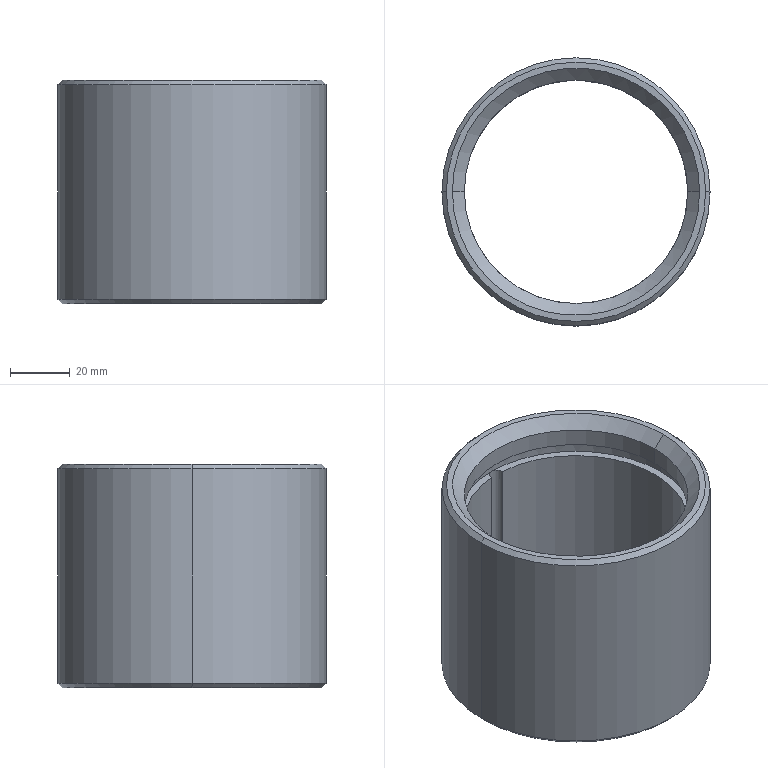Part | SolidWorks | features Chamfer 2, ICE 2, Extrusion 1 | 1 solid | 29 faces | box 90 x 90 x 75 mm | volume 139007 mm3 | cylinder 15 | cone 9 | plane 5 | commonest cylinder face diameters 5 x6 75 x5 80 x2 90 x2
STEP:
#1=CARTESIAN_POINT('',(-2.499,37.417,-36.));
#2=VERTEX_POINT('',#1);
#3=CARTESIAN_POINT('',(-2.5,37.5,-36.083));
#4=VERTEX_POINT('',#3);
#5=CARTESIAN_POINT('',(-2.499,37.417,-36.));
#6=CARTESIAN_POINT('',(-2.5,37.444,-36.028));
#7=CARTESIAN_POINT('',(-2.5,37.472,-36.056));
#8=CARTESIAN_POINT('',(-2.5,37.5,-36.083));
#9=B_SPLINE_CURVE_WITH_KNOTS('',3,(#5,#6,#7,#8),.UNSPECIFIED.,.F.,.F.,(4,4),(0.000000279,0.0001166),.UNSPECIFIED.);
#10=EDGE_CURVE('',#2,#4,#9,.T.);
#11=ORIENTED_EDGE('',*,*,#10,.T.);
#12=CARTESIAN_POINT('',(-2.5,37.5,23.));
#13=VERTEX_POINT('',#12);
#14=CARTESIAN_POINT('',(-2.5,37.5,-37.5));
#15=DIRECTION('',(0.,0.,1.));
#16=VECTOR('',#15,1000.);
#17=LINE('',#14,#16);
#18=EDGE_CURVE('',#4,#13,#17,.T.);
#19=ORIENTED_EDGE('',*,*,#18,.T.);
#20=CARTESIAN_POINT('',(-2.499,37.417,23.));
#21=VERTEX_POINT('',#20);
#22=CARTESIAN_POINT('',(0.,37.5,23.));
#23=DIRECTION('',(0.,0.,1.));
#24=DIRECTION('',(1.,0.,0.));
#25=AXIS2_PLACEMENT_3D('',#22,#23,#24);
#26=CIRCLE('',#25,2.5);
#27=EDGE_CURVE('',#13,#21,#26,.T.);
#28=ORIENTED_EDGE('',*,*,#27,.T.);
#29=CARTESIAN_POINT('',(-2.499,37.417,-37.5));
#30=DIRECTION('',(0.,0.,1.));
#31=VECTOR('',#30,1000.);
#32=LINE('',#29,#31);
#33=EDGE_CURVE('',#2,#21,#32,.T.);
#34=ORIENTED_EDGE('',*,*,#33,.F.);
#35=EDGE_LOOP('',(#11,#19,#28,#34));
#36=FACE_OUTER_BOUND('',#35,.T.);
#37=CARTESIAN_POINT('',(0.,37.5,-37.5));
#38=DIRECTION('',(0.,0.,1.));
#39=DIRECTION('',(1.,0.,0.));
#40=AXIS2_PLACEMENT_3D('',#37,#38,#39);
#41=CYLINDRICAL_SURFACE('',#40,2.5);
#42=ADVANCED_FACE('',(#36),#41,.F.);
#43=ORIENTED_EDGE('',*,*,#18,.F.);
#44=CARTESIAN_POINT('',(-2.039,38.947,-37.5));
#45=VERTEX_POINT('',#44);
#46=CARTESIAN_POINT('',(-2.5,37.5,-36.083));
#47=CARTESIAN_POINT('',(-2.5,37.748,-36.331));
#48=CARTESIAN_POINT('',(-2.464,37.994,-36.573));
#49=CARTESIAN_POINT('',(-2.314,38.479,-37.049));
#50=CARTESIAN_POINT('',(-2.199,38.72,-37.282));
#51=CARTESIAN_POINT('',(-2.039,38.947,-37.5));
#52=B_SPLINE_CURVE_WITH_KNOTS('',3,(#46,#47,#48,#49,#50,#51),.UNSPECIFIED.,.F.,.F.,(4,2,4),(0.0001166,0.001157,0.002198),.UNSPECIFIED.);
#53=EDGE_CURVE('',#4,#45,#52,.T.);
#54=ORIENTED_EDGE('',*,*,#53,.T.);
#55=CARTESIAN_POINT('',(2.039,38.947,-37.5));
#56=VERTEX_POINT('',#55);
#57=CARTESIAN_POINT('',(0.,37.5,-37.5));
#58=DIRECTION('',(0.,0.,1.));
#59=DIRECTION('',(-1.,0.,0.));
#60=AXIS2_PLACEMENT_3D('',#57,#58,#59);
#61=CIRCLE('',#60,2.5);
#62=EDGE_CURVE('',#56,#45,#61,.T.);
#63=ORIENTED_EDGE('',*,*,#62,.F.);
#64=CARTESIAN_POINT('',(2.5,37.5,-36.083));
#65=VERTEX_POINT('',#64);
#66=CARTESIAN_POINT('',(2.039,38.947,-37.5));
#67=CARTESIAN_POINT('',(2.199,38.721,-37.283));
#68=CARTESIAN_POINT('',(2.312,38.485,-37.054));
#69=CARTESIAN_POINT('',(2.463,37.998,-36.577));
#70=CARTESIAN_POINT('',(2.5,37.748,-36.331));
#71=CARTESIAN_POINT('',(2.5,37.5,-36.083));
#72=B_SPLINE_CURVE_WITH_KNOTS('',3,(#66,#67,#68,#69,#70,#71),.UNSPECIFIED.,.F.,.F.,(4,2,4),(0.00000032,0.001043,0.002085),.UNSPECIFIED.);
#73=EDGE_CURVE('',#56,#65,#72,.T.);
#74=ORIENTED_EDGE('',*,*,#73,.T.);
#75=CARTESIAN_POINT('',(2.5,37.5,23.));
#76=VERTEX_POINT('',#75);
#77=CARTESIAN_POINT('',(2.5,37.5,-37.5));
#78=DIRECTION('',(0.,0.,1.));
#79=VECTOR('',#78,1000.);
#80=LINE('',#77,#79);
#81=EDGE_CURVE('',#65,#76,#80,.T.);
#82=ORIENTED_EDGE('',*,*,#81,.T.);
#83=CARTESIAN_POINT('',(0.,40.,23.));
#84=VERTEX_POINT('',#83);
#85=CARTESIAN_POINT('',(0.,37.5,23.));
#86=DIRECTION('',(0.,0.,1.));
#87=DIRECTION('',(1.,0.,0.));
#88=AXIS2_PLACEMENT_3D('',#85,#86,#87);
#89=CIRCLE('',#88,2.5);
#90=EDGE_CURVE('',#76,#84,#89,.T.);
#91=ORIENTED_EDGE('',*,*,#90,.T.);
#92=CARTESIAN_POINT('',(0.,37.5,23.));
#93=DIRECTION('',(0.,0.,1.));
#94=DIRECTION('',(1.,0.,0.));
#95=AXIS2_PLACEMENT_3D('',#92,#93,#94);
#96=CIRCLE('',#95,2.5);
#97=EDGE_CURVE('',#84,#13,#96,.T.);
#98=ORIENTED_EDGE('',*,*,#97,.T.);
#99=EDGE_LOOP('',(#43,#54,#63,#74,#82,#91,#98));
#100=FACE_OUTER_BOUND('',#99,.T.);
#101=CARTESIAN_POINT('',(0.,37.5,-37.5));
#102=DIRECTION('',(0.,0.,1.));
#103=DIRECTION('',(1.,0.,0.));
#104=AXIS2_PLACEMENT_3D('',#101,#102,#103);
#105=CYLINDRICAL_SURFACE('',#104,2.5);
#106=ADVANCED_FACE('',(#100),#105,.F.);
#107=CARTESIAN_POINT('',(-2.039,-38.947,-37.5));
#108=VERTEX_POINT('',#107);
#109=CARTESIAN_POINT('',(-2.5,-37.5,-36.083));
#110=VERTEX_POINT('',#109);
#111=CARTESIAN_POINT('',(-2.039,-38.947,-37.5));
#112=CARTESIAN_POINT('',(-2.199,-38.721,-37.283));
#113=CARTESIAN_POINT('',(-2.312,-38.485,-37.054));
#114=CARTESIAN_POINT('',(-2.463,-37.998,-36.577));
#115=CARTESIAN_POINT('',(-2.5,-37.748,-36.331));
#116=CARTESIAN_POINT('',(-2.5,-37.5,-36.083));
#117=B_SPLINE_CURVE_WITH_KNOTS('',3,(#111,#112,#113,#114,#115,#116),.UNSPECIFIED.,.F.,.F.,(4,2,4),(0.00000032,0.001043,0.002085),.UNSPECIFIED.);
#118=EDGE_CURVE('',#108,#110,#117,.T.);
#119=ORIENTED_EDGE('',*,*,#118,.T.);
#120=CARTESIAN_POINT('',(-2.5,-37.5,23.));
#121=VERTEX_POINT('',#120);
#122=CARTESIAN_POINT('',(-2.5,-37.5,-37.5));
#123=DIRECTION('',(0.,0.,1.));
#124=VECTOR('',#123,1000.);
#125=LINE('',#122,#124);
#126=EDGE_CURVE('',#110,#121,#125,.T.);
#127=ORIENTED_EDGE('',*,*,#126,.T.);
#128=CARTESIAN_POINT('',(0.,-40.,23.));
#129=VERTEX_POINT('',#128);
#130=CARTESIAN_POINT('',(0.,-37.5,23.));
#131=DIRECTION('',(0.,0.,1.));
#132=DIRECTION('',(1.,0.,0.));
#133=AXIS2_PLACEMENT_3D('',#130,#131,#132);
#134=CIRCLE('',#133,2.5);
#135=EDGE_CURVE('',#121,#129,#134,.T.);
#136=ORIENTED_EDGE('',*,*,#135,.T.);
#137=CARTESIAN_POINT('',(2.5,-37.5,23.));
#138=VERTEX_POINT('',#137);
#139=CARTESIAN_POINT('',(0.,-37.5,23.));
#140=DIRECTION('',(0.,0.,1.));
#141=DIRECTION('',(1.,0.,0.));
#142=AXIS2_PLACEMENT_3D('',#139,#140,#141);
#143=CIRCLE('',#142,2.5);
#144=EDGE_CURVE('',#129,#138,#143,.T.);
#145=ORIENTED_EDGE('',*,*,#144,.T.);
#146=CARTESIAN_POINT('',(2.5,-37.5,-36.083));
#147=VERTEX_POINT('',#146);
#148=CARTESIAN_POINT('',(2.5,-37.5,-37.5));
#149=DIRECTION('',(0.,0.,1.));
#150=VECTOR('',#149,1000.);
#151=LINE('',#148,#150);
#152=EDGE_CURVE('',#147,#138,#151,.T.);
#153=ORIENTED_EDGE('',*,*,#152,.F.);
#154=CARTESIAN_POINT('',(2.039,-38.947,-37.5));
#155=VERTEX_POINT('',#154);
#156=CARTESIAN_POINT('',(2.5,-37.5,-36.083));
#157=CARTESIAN_POINT('',(2.5,-37.748,-36.331));
#158=CARTESIAN_POINT('',(2.464,-37.994,-36.573));
#159=CARTESIAN_POINT('',(2.314,-38.479,-37.049));
#160=CARTESIAN_POINT('',(2.199,-38.72,-37.282));
#161=CARTESIAN_POINT('',(2.039,-38.947,-37.5));
#162=B_SPLINE_CURVE_WITH_KNOTS('',3,(#156,#157,#158,#159,#160,#161),.UNSPECIFIED.,.F.,.F.,(4,2,4),(0.0001166,0.001157,0.002198),.UNSPECIFIED.);
#163=EDGE_CURVE('',#147,#155,#162,.T.);
#164=ORIENTED_EDGE('',*,*,#163,.T.);
#165=CARTESIAN_POINT('',(0.,-37.5,-37.5));
#166=DIRECTION('',(0.,0.,1.));
#167=DIRECTION('',(1.,0.,0.));
#168=AXIS2_PLACEMENT_3D('',#165,#166,#167);
#169=CIRCLE('',#168,2.5);
#170=EDGE_CURVE('',#108,#155,#169,.T.);
#171=ORIENTED_EDGE('',*,*,#170,.F.);
#172=EDGE_LOOP('',(#119,#127,#136,#145,#153,#164,#171));
#173=FACE_OUTER_BOUND('',#172,.T.);
#174=CARTESIAN_POINT('',(0.,-37.5,-37.5));
#175=DIRECTION('',(0.,0.,1.));
#176=DIRECTION('',(1.,0.,0.));
#177=AXIS2_PLACEMENT_3D('',#174,#175,#176);
#178=CYLINDRICAL_SURFACE('',#177,2.5);
#179=ADVANCED_FACE('',(#173),#178,.F.);
#180=CARTESIAN_POINT('',(2.499,-37.417,-36.));
#181=VERTEX_POINT('',#180);
#182=CARTESIAN_POINT('',(2.499,-37.417,-36.));
#183=CARTESIAN_POINT('',(2.5,-37.444,-36.028));
#184=CARTESIAN_POINT('',(2.5,-37.472,-36.056));
#185=CARTESIAN_POINT('',(2.5,-37.5,-36.083));
#186=B_SPLINE_CURVE_WITH_KNOTS('',3,(#182,#183,#184,#185),.UNSPECIFIED.,.F.,.F.,(4,4),(0.000000279,0.0001166),.UNSPECIFIED.);
#187=EDGE_CURVE('',#181,#147,#186,.T.);
#188=ORIENTED_EDGE('',*,*,#187,.T.);
#189=ORIENTED_EDGE('',*,*,#152,.T.);
#190=CARTESIAN_POINT('',(2.499,-37.417,23.));
#191=VERTEX_POINT('',#190);
#192=CARTESIAN_POINT('',(0.,-37.5,23.));
#193=DIRECTION('',(0.,0.,1.));
#194=DIRECTION('',(1.,0.,0.));
#195=AXIS2_PLACEMENT_3D('',#192,#193,#194);
#196=CIRCLE('',#195,2.5);
#197=EDGE_CURVE('',#138,#191,#196,.T.);
#198=ORIENTED_EDGE('',*,*,#197,.T.);
#199=CARTESIAN_POINT('',(2.499,-37.417,-37.5));
#200=DIRECTION('',(0.,0.,1.));
#201=VECTOR('',#200,1000.);
#202=LINE('',#199,#201);
#203=EDGE_CURVE('',#181,#191,#202,.T.);
#204=ORIENTED_EDGE('',*,*,#203,.F.);
#205=EDGE_LOOP('',(#188,#189,#198,#204));
#206=FACE_OUTER_BOUND('',#205,.T.);
#207=CARTESIAN_POINT('',(0.,-37.5,-37.5));
#208=DIRECTION('',(0.,0.,1.));
#209=DIRECTION('',(1.,0.,0.));
#210=AXIS2_PLACEMENT_3D('',#207,#208,#209);
#211=CYLINDRICAL_SURFACE('',#210,2.5);
#212=ADVANCED_FACE('',(#206),#211,.F.);
#213=CARTESIAN_POINT('',(-37.5,0.,33.5));
#214=VERTEX_POINT('',#213);
#215=CARTESIAN_POINT('',(37.5,0.,33.5));
#216=VERTEX_POINT('',#215);
#217=CARTESIAN_POINT('',(0.,0.,33.5));
#218=DIRECTION('',(0.,0.,1.));
#219=DIRECTION('',(1.,0.,0.));
#220=AXIS2_PLACEMENT_3D('',#217,#218,#219);
#221=CIRCLE('',#220,37.5);
#222=EDGE_CURVE('',#214,#216,#221,.T.);
#223=ORIENTED_EDGE('',*,*,#222,.F.);
#224=CARTESIAN_POINT('',(-41.5,0.,37.5));
#225=VERTEX_POINT('',#224);
#226=CARTESIAN_POINT('',(-37.5,0.,33.5));
#227=DIRECTION('',(-0.7071,0.,0.7071));
#228=VECTOR('',#227,1000.);
#229=LINE('',#226,#228);
#230=EDGE_CURVE('',#214,#225,#229,.T.);
#231=ORIENTED_EDGE('',*,*,#230,.T.);
#232=CARTESIAN_POINT('',(41.5,0.,37.5));
#233=VERTEX_POINT('',#232);
#234=CARTESIAN_POINT('',(0.,0.,37.5));
#235=DIRECTION('',(0.,0.,-1.));
#236=DIRECTION('',(1.,0.,0.));
#237=AXIS2_PLACEMENT_3D('',#234,#235,#236);
#238=CIRCLE('',#237,41.5);
#239=EDGE_CURVE('',#233,#225,#238,.T.);
#240=ORIENTED_EDGE('',*,*,#239,.F.);
#241=CARTESIAN_POINT('',(37.5,0.,33.5));
#242=DIRECTION('',(0.7071,0.,0.7071));
#243=VECTOR('',#242,1000.);
#244=LINE('',#241,#243);
#245=EDGE_CURVE('',#216,#233,#244,.T.);
#246=ORIENTED_EDGE('',*,*,#245,.F.);
#247=EDGE_LOOP('',(#223,#231,#240,#246));
#248=FACE_OUTER_BOUND('',#247,.T.);
#249=CARTESIAN_POINT('',(0.,0.,33.5));
#250=DIRECTION('',(0.,0.,1.));
#251=DIRECTION('',(1.,0.,0.));
#252=AXIS2_PLACEMENT_3D('',#249,#250,#251);
#253=CONICAL_SURFACE('',#252,37.5,0.7854);
#254=ADVANCED_FACE('',(#248),#253,.F.);
#255=CARTESIAN_POINT('',(43.5,0.,37.5));
#256=VERTEX_POINT('',#255);
#257=CARTESIAN_POINT('',(-43.5,0.,37.5));
#258=VERTEX_POINT('',#257);
#259=CARTESIAN_POINT('',(0.,0.,37.5));
#260=DIRECTION('',(0.,0.,1.));
#261=DIRECTION('',(1.,0.,0.));
#262=AXIS2_PLACEMENT_3D('',#259,#260,#261);
#263=CIRCLE('',#262,43.5);
#264=EDGE_CURVE('',#256,#258,#263,.T.);
#265=ORIENTED_EDGE('',*,*,#264,.F.);
#266=CARTESIAN_POINT('',(45.,0.,36.));
#267=VERTEX_POINT('',#266);
#268=CARTESIAN_POINT('',(43.5,0.,37.5));
#269=DIRECTION('',(0.7071,0.,-0.7071));
#270=VECTOR('',#269,1000.);
#271=LINE('',#268,#270);
#272=EDGE_CURVE('',#256,#267,#271,.T.);
#273=ORIENTED_EDGE('',*,*,#272,.T.);
#274=CARTESIAN_POINT('',(-45.,0.,36.));
#275=VERTEX_POINT('',#274);
#276=CARTESIAN_POINT('',(0.,0.,36.));
#277=DIRECTION('',(0.,0.,-1.));
#278=DIRECTION('',(1.,0.,0.));
#279=AXIS2_PLACEMENT_3D('',#276,#277,#278);
#280=CIRCLE('',#279,45.);
#281=EDGE_CURVE('',#275,#267,#280,.T.);
#282=ORIENTED_EDGE('',*,*,#281,.F.);
#283=CARTESIAN_POINT('',(-43.5,0.,37.5));
#284=DIRECTION('',(-0.7071,0.,-0.7071));
#285=VECTOR('',#284,1000.);
#286=LINE('',#283,#285);
#287=EDGE_CURVE('',#258,#275,#286,.T.);
#288=ORIENTED_EDGE('',*,*,#287,.F.);
#289=EDGE_LOOP('',(#265,#273,#282,#288));
#290=FACE_OUTER_BOUND('',#289,.T.);
#291=CARTESIAN_POINT('',(0.,0.,37.5));
#292=DIRECTION('',(0.,0.,-1.));
#293=DIRECTION('',(-1.,0.,0.));
#294=AXIS2_PLACEMENT_3D('',#291,#292,#293);
#295=CONICAL_SURFACE('',#294,43.5,0.7854);
#296=ADVANCED_FACE('',(#290),#295,.T.);
#297=CARTESIAN_POINT('',(-43.5,0.,-37.5));
#298=VERTEX_POINT('',#297);
#299=CARTESIAN_POINT('',(43.5,0.,-37.5));
#300=VERTEX_POINT('',#299);
#301=CARTESIAN_POINT('',(0.,0.,-37.5));
#302=DIRECTION('',(0.,0.,-1.));
#303=DIRECTION('',(1.,0.,0.));
#304=AXIS2_PLACEMENT_3D('',#301,#302,#303);
#305=CIRCLE('',#304,43.5);
#306=EDGE_CURVE('',#298,#300,#305,.T.);
#307=ORIENTED_EDGE('',*,*,#306,.F.);
#308=CARTESIAN_POINT('',(-45.,0.,-36.));
#309=VERTEX_POINT('',#308);
#310=CARTESIAN_POINT('',(-45.,0.,-36.));
#311=DIRECTION('',(-0.7071,0.,0.7071));
#312=VECTOR('',#311,1000.);
#313=LINE('',#310,#312);
#314=EDGE_CURVE('',#298,#309,#313,.T.);
#315=ORIENTED_EDGE('',*,*,#314,.T.);
#316=CARTESIAN_POINT('',(45.,0.,-36.));
#317=VERTEX_POINT('',#316);
#318=CARTESIAN_POINT('',(0.,0.,-36.));
#319=DIRECTION('',(0.,0.,1.));
#320=DIRECTION('',(1.,0.,0.));
#321=AXIS2_PLACEMENT_3D('',#318,#319,#320);
#322=CIRCLE('',#321,45.);
#323=EDGE_CURVE('',#317,#309,#322,.T.);
#324=ORIENTED_EDGE('',*,*,#323,.F.);
#325=CARTESIAN_POINT('',(45.,0.,-36.));
#326=DIRECTION('',(0.7071,0.,0.7071));
#327=VECTOR('',#326,1000.);
#328=LINE('',#325,#327);
#329=EDGE_CURVE('',#300,#317,#328,.T.);
#330=ORIENTED_EDGE('',*,*,#329,.F.);
#331=EDGE_LOOP('',(#307,#315,#324,#330));
#332=FACE_OUTER_BOUND('',#331,.T.);
#333=CARTESIAN_POINT('',(0.,0.,-36.));
#334=DIRECTION('',(0.,0.,1.));
#335=DIRECTION('',(1.,0.,0.));
#336=AXIS2_PLACEMENT_3D('',#333,#334,#335);
#337=CONICAL_SURFACE('',#336,45.,0.7854);
#338=ADVANCED_FACE('',(#332),#337,.T.);
#339=CARTESIAN_POINT('',(-37.5,0.,-36.));
#340=VERTEX_POINT('',#339);
#341=CARTESIAN_POINT('',(0.,0.,-36.));
#342=DIRECTION('',(0.,0.,-1.));
#343=DIRECTION('',(1.,0.,0.));
#344=AXIS2_PLACEMENT_3D('',#341,#342,#343);
#345=CIRCLE('',#344,37.5);
#346=EDGE_CURVE('',#340,#2,#345,.T.);
#347=ORIENTED_EDGE('',*,*,#346,.F.);
#348=CARTESIAN_POINT('',(-39.,0.,-37.5));
#349=VERTEX_POINT('',#348);
#350=CARTESIAN_POINT('',(-39.,0.,-37.5));
#351=DIRECTION('',(-0.7071,0.,-0.7071));
#352=VECTOR('',#351,1000.);
#353=LINE('',#350,#352);
#354=EDGE_CURVE('',#340,#349,#353,.T.);
#355=ORIENTED_EDGE('',*,*,#354,.T.);
#356=CARTESIAN_POINT('',(0.,0.,-37.5));
#357=DIRECTION('',(0.,0.,1.));
#358=DIRECTION('',(1.,0.,0.));
#359=AXIS2_PLACEMENT_3D('',#356,#357,#358);
#360=CIRCLE('',#359,39.);
#361=EDGE_CURVE('',#45,#349,#360,.T.);
#362=ORIENTED_EDGE('',*,*,#361,.F.);
#363=ORIENTED_EDGE('',*,*,#53,.F.);
#364=ORIENTED_EDGE('',*,*,#10,.F.);
#365=EDGE_LOOP('',(#347,#355,#362,#363,#364));
#366=FACE_OUTER_BOUND('',#365,.T.);
#367=CARTESIAN_POINT('',(0.,0.,-37.5));
#368=DIRECTION('',(0.,0.,-1.));
#369=DIRECTION('',(-1.,0.,0.));
#370=AXIS2_PLACEMENT_3D('',#367,#368,#369);
#371=CONICAL_SURFACE('',#370,39.,0.7854);
#372=ADVANCED_FACE('',(#366),#371,.F.);
#373=CARTESIAN_POINT('',(-40.,0.,23.));
#374=VERTEX_POINT('',#373);
#375=CARTESIAN_POINT('',(0.,0.,23.));
#376=DIRECTION('',(0.,0.,1.));
#377=DIRECTION('',(1.,0.,0.));
#378=AXIS2_PLACEMENT_3D('',#375,#376,#377);
#379=CIRCLE('',#378,40.);
#380=EDGE_CURVE('',#374,#129,#379,.T.);
#381=ORIENTED_EDGE('',*,*,#380,.F.);
#382=CARTESIAN_POINT('',(-40.,0.,27.5));
#383=VERTEX_POINT('',#382);
#384=CARTESIAN_POINT('',(-40.,0.,23.));
#385=DIRECTION('',(0.,0.,1.));
#386=VECTOR('',#385,1000.);
#387=LINE('',#384,#386);
#388=EDGE_CURVE('',#374,#383,#387,.T.);
#389=ORIENTED_EDGE('',*,*,#388,.T.);
#390=CARTESIAN_POINT('',(40.,0.,27.5));
#391=VERTEX_POINT('',#390);
#392=CARTESIAN_POINT('',(0.,0.,27.5));
#393=DIRECTION('',(0.,0.,1.));
#394=DIRECTION('',(1.,0.,0.));
#395=AXIS2_PLACEMENT_3D('',#392,#393,#394);
#396=CIRCLE('',#395,40.);
#397=EDGE_CURVE('',#383,#391,#396,.T.);
#398=ORIENTED_EDGE('',*,*,#397,.T.);
#399=CARTESIAN_POINT('',(40.,0.,23.));
#400=VERTEX_POINT('',#399);
#401=CARTESIAN_POINT('',(40.,0.,23.));
#402=DIRECTION('',(0.,0.,1.));
#403=VECTOR('',#402,1000.);
#404=LINE('',#401,#403);
#405=EDGE_CURVE('',#400,#391,#404,.T.);
#406=ORIENTED_EDGE('',*,*,#405,.F.);
#407=CARTESIAN_POINT('',(0.,0.,23.));
#408=DIRECTION('',(0.,0.,1.));
#409=DIRECTION('',(1.,0.,0.));
#410=AXIS2_PLACEMENT_3D('',#407,#408,#409);
#411=CIRCLE('',#410,40.);
#412=EDGE_CURVE('',#129,#400,#411,.T.);
#413=ORIENTED_EDGE('',*,*,#412,.F.);
#414=EDGE_LOOP('',(#381,#389,#398,#406,#413));
#415=FACE_OUTER_BOUND('',#414,.T.);
#416=CARTESIAN_POINT('',(0.,0.,23.));
#417=DIRECTION('',(0.,0.,1.));
#418=DIRECTION('',(1.,0.,0.));
#419=AXIS2_PLACEMENT_3D('',#416,#417,#418);
#420=CYLINDRICAL_SURFACE('',#419,40.);
#421=ADVANCED_FACE('',(#415),#420,.F.);
#422=ORIENTED_EDGE('',*,*,#222,.T.);
#423=CARTESIAN_POINT('',(37.5,0.,27.5));
#424=VERTEX_POINT('',#423);
#425=CARTESIAN_POINT('',(37.5,0.,37.5));
#426=DIRECTION('',(0.,0.,-1.));
#427=VECTOR('',#426,1000.);
#428=LINE('',#425,#427);
#429=EDGE_CURVE('',#216,#424,#428,.T.);
#430=ORIENTED_EDGE('',*,*,#429,.T.);
#431=CARTESIAN_POINT('',(-37.5,0.,27.5));
#432=VERTEX_POINT('',#431);
#433=CARTESIAN_POINT('',(0.,0.,27.5));
#434=DIRECTION('',(0.,0.,1.));
#435=DIRECTION('',(1.,0.,0.));
#436=AXIS2_PLACEMENT_3D('',#433,#434,#435);
#437=CIRCLE('',#436,37.5);
#438=EDGE_CURVE('',#432,#424,#437,.T.);
#439=ORIENTED_EDGE('',*,*,#438,.F.);
#440=CARTESIAN_POINT('',(-37.5,0.,37.5));
#441=DIRECTION('',(0.,0.,-1.));
#442=VECTOR('',#441,1000.);
#443=LINE('',#440,#442);
#444=EDGE_CURVE('',#214,#432,#443,.T.);
#445=ORIENTED_EDGE('',*,*,#444,.F.);
#446=EDGE_LOOP('',(#422,#430,#439,#445));
#447=FACE_OUTER_BOUND('',#446,.T.);
#448=CARTESIAN_POINT('',(0.,0.,37.5));
#449=DIRECTION('',(0.,0.,-1.));
#450=DIRECTION('',(-1.,0.,0.));
#451=AXIS2_PLACEMENT_3D('',#448,#449,#450);
#452=CYLINDRICAL_SURFACE('',#451,37.5);
#453=ADVANCED_FACE('',(#447),#452,.F.);
#454=ORIENTED_EDGE('',*,*,#281,.T.);
#455=CARTESIAN_POINT('',(45.,0.,37.5));
#456=DIRECTION('',(0.,0.,-1.));
#457=VECTOR('',#456,1000.);
#458=LINE('',#455,#457);
#459=EDGE_CURVE('',#267,#317,#458,.T.);
#460=ORIENTED_EDGE('',*,*,#459,.T.);
#461=ORIENTED_EDGE('',*,*,#323,.T.);
#462=CARTESIAN_POINT('',(-45.,0.,37.5));
#463=DIRECTION('',(0.,0.,-1.));
#464=VECTOR('',#463,1000.);
#465=LINE('',#462,#464);
#466=EDGE_CURVE('',#275,#309,#465,.T.);
#467=ORIENTED_EDGE('',*,*,#466,.F.);
#468=EDGE_LOOP('',(#454,#460,#461,#467));
#469=FACE_OUTER_BOUND('',#468,.T.);
#470=CARTESIAN_POINT('',(0.,0.,37.5));
#471=DIRECTION('',(0.,0.,-1.));
#472=DIRECTION('',(-1.,0.,0.));
#473=AXIS2_PLACEMENT_3D('',#470,#471,#472);
#474=CYLINDRICAL_SURFACE('',#473,45.);
#475=ADVANCED_FACE('',(#469),#474,.T.);
#476=CARTESIAN_POINT('',(-37.5,0.,23.));
#477=VERTEX_POINT('',#476);
#478=CARTESIAN_POINT('',(0.,0.,23.));
#479=DIRECTION('',(0.,0.,1.));
#480=DIRECTION('',(1.,0.,0.));
#481=AXIS2_PLACEMENT_3D('',#478,#479,#480);
#482=CIRCLE('',#481,37.5);
#483=EDGE_CURVE('',#21,#477,#482,.T.);
#484=ORIENTED_EDGE('',*,*,#483,.T.);
#485=CARTESIAN_POINT('',(-37.5,0.,37.5));
#486=DIRECTION('',(0.,0.,-1.));
#487=VECTOR('',#486,1000.);
#488=LINE('',#485,#487);
#489=EDGE_CURVE('',#477,#340,#488,.T.);
#490=ORIENTED_EDGE('',*,*,#489,.T.);
#491=ORIENTED_EDGE('',*,*,#346,.T.);
#492=ORIENTED_EDGE('',*,*,#33,.T.);
#493=EDGE_LOOP('',(#484,#490,#491,#492));
#494=FACE_OUTER_BOUND('',#493,.T.);
#495=CARTESIAN_POINT('',(0.,0.,37.5));
#496=DIRECTION('',(0.,0.,-1.));
#497=DIRECTION('',(-1.,0.,0.));
#498=AXIS2_PLACEMENT_3D('',#495,#496,#497);
#499=CYLINDRICAL_SURFACE('',#498,37.5);
#500=ADVANCED_FACE('',(#494),#499,.F.);
#501=CARTESIAN_POINT('',(2.499,37.417,-36.));
#502=VERTEX_POINT('',#501);
#503=CARTESIAN_POINT('',(2.499,37.417,23.));
#504=VERTEX_POINT('',#503);
#505=CARTESIAN_POINT('',(2.499,37.417,-37.5));
#506=DIRECTION('',(0.,0.,1.));
#507=VECTOR('',#506,1000.);
#508=LINE('',#505,#507);
#509=EDGE_CURVE('',#502,#504,#508,.T.);
#510=ORIENTED_EDGE('',*,*,#509,.F.);
#511=CARTESIAN_POINT('',(0.,0.,-36.));
#512=DIRECTION('',(0.,0.,-1.));
#513=DIRECTION('',(1.,0.,0.));
#514=AXIS2_PLACEMENT_3D('',#511,#512,#513);
#515=CIRCLE('',#514,37.5);
#516=EDGE_CURVE('',#502,#181,#515,.T.);
#517=ORIENTED_EDGE('',*,*,#516,.T.);
#518=ORIENTED_EDGE('',*,*,#203,.T.);
#519=CARTESIAN_POINT('',(0.,0.,23.));
#520=DIRECTION('',(0.,0.,1.));
#521=DIRECTION('',(1.,0.,0.));
#522=AXIS2_PLACEMENT_3D('',#519,#520,#521);
#523=CIRCLE('',#522,37.5);
#524=EDGE_CURVE('',#191,#504,#523,.T.);
#525=ORIENTED_EDGE('',*,*,#524,.T.);
#526=EDGE_LOOP('',(#510,#517,#518,#525));
#527=FACE_OUTER_BOUND('',#526,.T.);
#528=CARTESIAN_POINT('',(0.,0.,37.5));
#529=DIRECTION('',(0.,0.,-1.));
#530=DIRECTION('',(-1.,0.,0.));
#531=AXIS2_PLACEMENT_3D('',#528,#529,#530);
#532=CYLINDRICAL_SURFACE('',#531,37.5);
#533=ADVANCED_FACE('',(#527),#532,.F.);
#534=ORIENTED_EDGE('',*,*,#97,.F.);
#535=CARTESIAN_POINT('',(0.,0.,23.));
#536=DIRECTION('',(0.,0.,1.));
#537=DIRECTION('',(1.,0.,0.));
#538=AXIS2_PLACEMENT_3D('',#535,#536,#537);
#539=CIRCLE('',#538,40.);
#540=EDGE_CURVE('',#84,#374,#539,.T.);
#541=ORIENTED_EDGE('',*,*,#540,.T.);
#542=ORIENTED_EDGE('',*,*,#380,.T.);
#543=ORIENTED_EDGE('',*,*,#135,.F.);
#544=CARTESIAN_POINT('',(-2.499,-37.417,23.));
#545=VERTEX_POINT('',#544);
#546=CARTESIAN_POINT('',(0.,-37.5,23.));
#547=DIRECTION('',(0.,0.,1.));
#548=DIRECTION('',(1.,0.,0.));
#549=AXIS2_PLACEMENT_3D('',#546,#547,#548);
#550=CIRCLE('',#549,2.5);
#551=EDGE_CURVE('',#545,#121,#550,.T.);
#552=ORIENTED_EDGE('',*,*,#551,.F.);
#553=CARTESIAN_POINT('',(0.,0.,23.));
#554=DIRECTION('',(0.,0.,1.));
#555=DIRECTION('',(1.,0.,0.));
#556=AXIS2_PLACEMENT_3D('',#553,#554,#555);
#557=CIRCLE('',#556,37.5);
#558=EDGE_CURVE('',#477,#545,#557,.T.);
#559=ORIENTED_EDGE('',*,*,#558,.F.);
#560=ORIENTED_EDGE('',*,*,#483,.F.);
#561=ORIENTED_EDGE('',*,*,#27,.F.);
#562=EDGE_LOOP('',(#534,#541,#542,#543,#552,#559,#560,#561));
#563=FACE_OUTER_BOUND('',#562,.T.);
#564=CARTESIAN_POINT('',(0.,0.,23.));
#565=DIRECTION('',(0.,0.,1.));
#566=DIRECTION('',(1.,0.,0.));
#567=AXIS2_PLACEMENT_3D('',#564,#565,#566);
#568=PLANE('',#567);
#569=ADVANCED_FACE('',(#563),#568,.T.);
#570=ORIENTED_EDGE('',*,*,#73,.F.);
#571=CARTESIAN_POINT('',(0.,0.,-37.5));
#572=DIRECTION('',(0.,0.,1.));
#573=DIRECTION('',(1.,0.,0.));
#574=AXIS2_PLACEMENT_3D('',#571,#572,#573);
#575=CIRCLE('',#574,39.);
#576=EDGE_CURVE('',#155,#56,#575,.T.);
#577=ORIENTED_EDGE('',*,*,#576,.F.);
#578=ORIENTED_EDGE('',*,*,#163,.F.);
#579=ORIENTED_EDGE('',*,*,#187,.F.);
#580=ORIENTED_EDGE('',*,*,#516,.F.);
#581=CARTESIAN_POINT('',(2.5,37.5,-36.083));
#582=CARTESIAN_POINT('',(2.5,37.472,-36.056));
#583=CARTESIAN_POINT('',(2.5,37.444,-36.028));
#584=CARTESIAN_POINT('',(2.499,37.417,-36.));
#585=B_SPLINE_CURVE_WITH_KNOTS('',3,(#581,#582,#583,#584),.UNSPECIFIED.,.F.,.F.,(4,4),(0.002085,0.002202),.UNSPECIFIED.);
#586=EDGE_CURVE('',#65,#502,#585,.T.);
#587=ORIENTED_EDGE('',*,*,#586,.F.);
#588=EDGE_LOOP('',(#570,#577,#578,#579,#580,#587));
#589=FACE_OUTER_BOUND('',#588,.T.);
#590=CARTESIAN_POINT('',(0.,0.,-37.5));
#591=DIRECTION('',(0.,0.,-1.));
#592=DIRECTION('',(-1.,0.,0.));
#593=AXIS2_PLACEMENT_3D('',#590,#591,#592);
#594=CONICAL_SURFACE('',#593,39.,0.7854);
#595=ADVANCED_FACE('',(#589),#594,.F.);
#596=ORIENTED_EDGE('',*,*,#489,.F.);
#597=ORIENTED_EDGE('',*,*,#558,.T.);
#598=CARTESIAN_POINT('',(-2.499,-37.417,-36.));
#599=VERTEX_POINT('',#598);
#600=CARTESIAN_POINT('',(-2.499,-37.417,-37.5));
#601=DIRECTION('',(0.,0.,1.));
#602=VECTOR('',#601,1000.);
#603=LINE('',#600,#602);
#604=EDGE_CURVE('',#599,#545,#603,.T.);
#605=ORIENTED_EDGE('',*,*,#604,.F.);
#606=CARTESIAN_POINT('',(0.,0.,-36.));
#607=DIRECTION('',(0.,0.,-1.));
#608=DIRECTION('',(1.,0.,0.));
#609=AXIS2_PLACEMENT_3D('',#606,#607,#608);
#610=CIRCLE('',#609,37.5);
#611=EDGE_CURVE('',#599,#340,#610,.T.);
#612=ORIENTED_EDGE('',*,*,#611,.T.);
#613=EDGE_LOOP('',(#596,#597,#605,#612));
#614=FACE_OUTER_BOUND('',#613,.T.);
#615=CARTESIAN_POINT('',(0.,0.,37.5));
#616=DIRECTION('',(0.,0.,-1.));
#617=DIRECTION('',(-1.,0.,0.));
#618=AXIS2_PLACEMENT_3D('',#615,#616,#617);
#619=CYLINDRICAL_SURFACE('',#618,37.5);
#620=ADVANCED_FACE('',(#614),#619,.F.);
#621=ORIENTED_EDGE('',*,*,#239,.T.);
#622=CARTESIAN_POINT('',(0.,0.,37.5));
#623=DIRECTION('',(0.,0.,-1.));
#624=DIRECTION('',(1.,0.,0.));
#625=AXIS2_PLACEMENT_3D('',#622,#623,#624);
#626=CIRCLE('',#625,41.5);
#627=EDGE_CURVE('',#225,#233,#626,.T.);
#628=ORIENTED_EDGE('',*,*,#627,.T.);
#629=EDGE_LOOP('',(#621,#628));
#630=FACE_BOUND('',#629,.T.);
#631=CARTESIAN_POINT('',(0.,0.,37.5));
#632=DIRECTION('',(0.,0.,1.));
#633=DIRECTION('',(1.,0.,0.));
#634=AXIS2_PLACEMENT_3D('',#631,#632,#633);
#635=CIRCLE('',#634,43.5);
#636=EDGE_CURVE('',#258,#256,#635,.T.);
#637=ORIENTED_EDGE('',*,*,#636,.T.);
#638=ORIENTED_EDGE('',*,*,#264,.T.);
#639=EDGE_LOOP('',(#637,#638));
#640=FACE_OUTER_BOUND('',#639,.T.);
#641=CARTESIAN_POINT('',(0.,0.,37.5));
#642=DIRECTION('',(0.,0.,1.));
#643=DIRECTION('',(1.,0.,0.));
#644=AXIS2_PLACEMENT_3D('',#641,#642,#643);
#645=PLANE('',#644);
#646=ADVANCED_FACE('',(#630,#640),#645,.T.);
#647=ORIENTED_EDGE('',*,*,#576,.T.);
#648=ORIENTED_EDGE('',*,*,#62,.T.);
#649=ORIENTED_EDGE('',*,*,#361,.T.);
#650=CARTESIAN_POINT('',(0.,0.,-37.5));
#651=DIRECTION('',(0.,0.,1.));
#652=DIRECTION('',(1.,0.,0.));
#653=AXIS2_PLACEMENT_3D('',#650,#651,#652);
#654=CIRCLE('',#653,39.);
#655=EDGE_CURVE('',#349,#108,#654,.T.);
#656=ORIENTED_EDGE('',*,*,#655,.T.);
#657=ORIENTED_EDGE('',*,*,#170,.T.);
#658=EDGE_LOOP('',(#647,#648,#649,#656,#657));
#659=FACE_BOUND('',#658,.T.);
#660=CARTESIAN_POINT('',(0.,0.,-37.5));
#661=DIRECTION('',(0.,0.,-1.));
#662=DIRECTION('',(1.,0.,0.));
#663=AXIS2_PLACEMENT_3D('',#660,#661,#662);
#664=CIRCLE('',#663,43.5);
#665=EDGE_CURVE('',#300,#298,#664,.T.);
#666=ORIENTED_EDGE('',*,*,#665,.T.);
#667=ORIENTED_EDGE('',*,*,#306,.T.);
#668=EDGE_LOOP('',(#666,#667));
#669=FACE_OUTER_BOUND('',#668,.T.);
#670=CARTESIAN_POINT('',(0.,0.,-37.5));
#671=DIRECTION('',(0.,0.,1.));
#672=DIRECTION('',(1.,0.,0.));
#673=AXIS2_PLACEMENT_3D('',#670,#671,#672);
#674=PLANE('',#673);
#675=ADVANCED_FACE('',(#659,#669),#674,.F.);
#676=ORIENTED_EDGE('',*,*,#459,.F.);
#677=CARTESIAN_POINT('',(0.,0.,36.));
#678=DIRECTION('',(0.,0.,-1.));
#679=DIRECTION('',(1.,0.,0.));
#680=AXIS2_PLACEMENT_3D('',#677,#678,#679);
#681=CIRCLE('',#680,45.);
#682=EDGE_CURVE('',#267,#275,#681,.T.);
#683=ORIENTED_EDGE('',*,*,#682,.T.);
#684=ORIENTED_EDGE('',*,*,#466,.T.);
#685=CARTESIAN_POINT('',(0.,0.,-36.));
#686=DIRECTION('',(0.,0.,1.));
#687=DIRECTION('',(1.,0.,0.));
#688=AXIS2_PLACEMENT_3D('',#685,#686,#687);
#689=CIRCLE('',#688,45.);
#690=EDGE_CURVE('',#309,#317,#689,.T.);
#691=ORIENTED_EDGE('',*,*,#690,.T.);
#692=EDGE_LOOP('',(#676,#683,#684,#691));
#693=FACE_OUTER_BOUND('',#692,.T.);
#694=CARTESIAN_POINT('',(0.,0.,37.5));
#695=DIRECTION('',(0.,0.,-1.));
#696=DIRECTION('',(-1.,0.,0.));
#697=AXIS2_PLACEMENT_3D('',#694,#695,#696);
#698=CYLINDRICAL_SURFACE('',#697,45.);
#699=ADVANCED_FACE('',(#693),#698,.T.);
#700=ORIENTED_EDGE('',*,*,#429,.F.);
#701=CARTESIAN_POINT('',(0.,0.,33.5));
#702=DIRECTION('',(0.,0.,1.));
#703=DIRECTION('',(1.,0.,0.));
#704=AXIS2_PLACEMENT_3D('',#701,#702,#703);
#705=CIRCLE('',#704,37.5);
#706=EDGE_CURVE('',#216,#214,#705,.T.);
#707=ORIENTED_EDGE('',*,*,#706,.T.);
#708=ORIENTED_EDGE('',*,*,#444,.T.);
#709=CARTESIAN_POINT('',(0.,0.,27.5));
#710=DIRECTION('',(0.,0.,1.));
#711=DIRECTION('',(1.,0.,0.));
#712=AXIS2_PLACEMENT_3D('',#709,#710,#711);
#713=CIRCLE('',#712,37.5);
#714=EDGE_CURVE('',#424,#432,#713,.T.);
#715=ORIENTED_EDGE('',*,*,#714,.F.);
#716=EDGE_LOOP('',(#700,#707,#708,#715));
#717=FACE_OUTER_BOUND('',#716,.T.);
#718=CARTESIAN_POINT('',(0.,0.,37.5));
#719=DIRECTION('',(0.,0.,-1.));
#720=DIRECTION('',(-1.,0.,0.));
#721=AXIS2_PLACEMENT_3D('',#718,#719,#720);
#722=CYLINDRICAL_SURFACE('',#721,37.5);
#723=ADVANCED_FACE('',(#717),#722,.F.);
#724=ORIENTED_EDGE('',*,*,#388,.F.);
#725=ORIENTED_EDGE('',*,*,#540,.F.);
#726=CARTESIAN_POINT('',(0.,0.,23.));
#727=DIRECTION('',(0.,0.,1.));
#728=DIRECTION('',(1.,0.,0.));
#729=AXIS2_PLACEMENT_3D('',#726,#727,#728);
#730=CIRCLE('',#729,40.);
#731=EDGE_CURVE('',#400,#84,#730,.T.);
#732=ORIENTED_EDGE('',*,*,#731,.F.);
#733=ORIENTED_EDGE('',*,*,#405,.T.);
#734=CARTESIAN_POINT('',(0.,0.,27.5));
#735=DIRECTION('',(0.,0.,1.));
#736=DIRECTION('',(1.,0.,0.));
#737=AXIS2_PLACEMENT_3D('',#734,#735,#736);
#738=CIRCLE('',#737,40.);
#739=EDGE_CURVE('',#391,#383,#738,.T.);
#740=ORIENTED_EDGE('',*,*,#739,.T.);
#741=EDGE_LOOP('',(#724,#725,#732,#733,#740));
#742=FACE_OUTER_BOUND('',#741,.T.);
#743=CARTESIAN_POINT('',(0.,0.,23.));
#744=DIRECTION('',(0.,0.,1.));
#745=DIRECTION('',(1.,0.,0.));
#746=AXIS2_PLACEMENT_3D('',#743,#744,#745);
#747=CYLINDRICAL_SURFACE('',#746,40.);
#748=ADVANCED_FACE('',(#742),#747,.F.);
#749=CARTESIAN_POINT('',(0.,37.5,23.));
#750=DIRECTION('',(0.,0.,1.));
#751=DIRECTION('',(1.,0.,0.));
#752=AXIS2_PLACEMENT_3D('',#749,#750,#751);
#753=CIRCLE('',#752,2.5);
#754=EDGE_CURVE('',#504,#76,#753,.T.);
#755=ORIENTED_EDGE('',*,*,#754,.F.);
#756=ORIENTED_EDGE('',*,*,#524,.F.);
#757=ORIENTED_EDGE('',*,*,#197,.F.);
#758=ORIENTED_EDGE('',*,*,#144,.F.);
#759=ORIENTED_EDGE('',*,*,#412,.T.);
#760=ORIENTED_EDGE('',*,*,#731,.T.);
#761=ORIENTED_EDGE('',*,*,#90,.F.);
#762=EDGE_LOOP('',(#755,#756,#757,#758,#759,#760,#761));
#763=FACE_OUTER_BOUND('',#762,.T.);
#764=CARTESIAN_POINT('',(0.,0.,23.));
#765=DIRECTION('',(0.,0.,1.));
#766=DIRECTION('',(1.,0.,0.));
#767=AXIS2_PLACEMENT_3D('',#764,#765,#766);
#768=PLANE('',#767);
#769=ADVANCED_FACE('',(#763),#768,.T.);
#770=ORIENTED_EDGE('',*,*,#438,.T.);
#771=ORIENTED_EDGE('',*,*,#714,.T.);
#772=EDGE_LOOP('',(#770,#771));
#773=FACE_BOUND('',#772,.T.);
#774=ORIENTED_EDGE('',*,*,#739,.F.);
#775=ORIENTED_EDGE('',*,*,#397,.F.);
#776=EDGE_LOOP('',(#774,#775));
#777=FACE_OUTER_BOUND('',#776,.T.);
#778=CARTESIAN_POINT('',(0.,0.,27.5));
#779=DIRECTION('',(0.,0.,1.));
#780=DIRECTION('',(1.,0.,0.));
#781=AXIS2_PLACEMENT_3D('',#778,#779,#780);
#782=PLANE('',#781);
#783=ADVANCED_FACE('',(#773,#777),#782,.F.);
#784=ORIENTED_EDGE('',*,*,#354,.F.);
#785=ORIENTED_EDGE('',*,*,#611,.F.);
#786=CARTESIAN_POINT('',(-2.5,-37.5,-36.083));
#787=CARTESIAN_POINT('',(-2.5,-37.472,-36.056));
#788=CARTESIAN_POINT('',(-2.5,-37.444,-36.028));
#789=CARTESIAN_POINT('',(-2.499,-37.417,-36.));
#790=B_SPLINE_CURVE_WITH_KNOTS('',3,(#786,#787,#788,#789),.UNSPECIFIED.,.F.,.F.,(4,4),(0.002085,0.002202),.UNSPECIFIED.);
#791=EDGE_CURVE('',#110,#599,#790,.T.);
#792=ORIENTED_EDGE('',*,*,#791,.F.);
#793=ORIENTED_EDGE('',*,*,#118,.F.);
#794=ORIENTED_EDGE('',*,*,#655,.F.);
#795=EDGE_LOOP('',(#784,#785,#792,#793,#794));
#796=FACE_OUTER_BOUND('',#795,.T.);
#797=CARTESIAN_POINT('',(0.,0.,-37.5));
#798=DIRECTION('',(0.,0.,-1.));
#799=DIRECTION('',(-1.,0.,0.));
#800=AXIS2_PLACEMENT_3D('',#797,#798,#799);
#801=CONICAL_SURFACE('',#800,39.,0.7854);
#802=ADVANCED_FACE('',(#796),#801,.F.);
#803=ORIENTED_EDGE('',*,*,#314,.F.);
#804=ORIENTED_EDGE('',*,*,#665,.F.);
#805=ORIENTED_EDGE('',*,*,#329,.T.);
#806=ORIENTED_EDGE('',*,*,#690,.F.);
#807=EDGE_LOOP('',(#803,#804,#805,#806));
#808=FACE_OUTER_BOUND('',#807,.T.);
#809=CARTESIAN_POINT('',(0.,0.,-36.));
#810=DIRECTION('',(0.,0.,1.));
#811=DIRECTION('',(1.,0.,0.));
#812=AXIS2_PLACEMENT_3D('',#809,#810,#811);
#813=CONICAL_SURFACE('',#812,45.,0.7854);
#814=ADVANCED_FACE('',(#808),#813,.T.);
#815=ORIENTED_EDGE('',*,*,#272,.F.);
#816=ORIENTED_EDGE('',*,*,#636,.F.);
#817=ORIENTED_EDGE('',*,*,#287,.T.);
#818=ORIENTED_EDGE('',*,*,#682,.F.);
#819=EDGE_LOOP('',(#815,#816,#817,#818));
#820=FACE_OUTER_BOUND('',#819,.T.);
#821=CARTESIAN_POINT('',(0.,0.,37.5));
#822=DIRECTION('',(0.,0.,-1.));
#823=DIRECTION('',(-1.,0.,0.));
#824=AXIS2_PLACEMENT_3D('',#821,#822,#823);
#825=CONICAL_SURFACE('',#824,43.5,0.7854);
#826=ADVANCED_FACE('',(#820),#825,.T.);
#827=ORIENTED_EDGE('',*,*,#230,.F.);
#828=ORIENTED_EDGE('',*,*,#706,.F.);
#829=ORIENTED_EDGE('',*,*,#245,.T.);
#830=ORIENTED_EDGE('',*,*,#627,.F.);
#831=EDGE_LOOP('',(#827,#828,#829,#830));
#832=FACE_OUTER_BOUND('',#831,.T.);
#833=CARTESIAN_POINT('',(0.,0.,33.5));
#834=DIRECTION('',(0.,0.,1.));
#835=DIRECTION('',(1.,0.,0.));
#836=AXIS2_PLACEMENT_3D('',#833,#834,#835);
#837=CONICAL_SURFACE('',#836,37.5,0.7854);
#838=ADVANCED_FACE('',(#832),#837,.F.);
#839=ORIENTED_EDGE('',*,*,#126,.F.);
#840=ORIENTED_EDGE('',*,*,#791,.T.);
#841=ORIENTED_EDGE('',*,*,#604,.T.);
#842=ORIENTED_EDGE('',*,*,#551,.T.);
#843=EDGE_LOOP('',(#839,#840,#841,#842));
#844=FACE_OUTER_BOUND('',#843,.T.);
#845=CARTESIAN_POINT('',(0.,-37.5,-37.5));
#846=DIRECTION('',(0.,0.,1.));
#847=DIRECTION('',(1.,0.,0.));
#848=AXIS2_PLACEMENT_3D('',#845,#846,#847);
#849=CYLINDRICAL_SURFACE('',#848,2.5);
#850=ADVANCED_FACE('',(#844),#849,.F.);
#851=ORIENTED_EDGE('',*,*,#81,.F.);
#852=ORIENTED_EDGE('',*,*,#586,.T.);
#853=ORIENTED_EDGE('',*,*,#509,.T.);
#854=ORIENTED_EDGE('',*,*,#754,.T.);
#855=EDGE_LOOP('',(#851,#852,#853,#854));
#856=FACE_OUTER_BOUND('',#855,.T.);
#857=CARTESIAN_POINT('',(0.,37.5,-37.5));
#858=DIRECTION('',(0.,0.,1.));
#859=DIRECTION('',(1.,0.,0.));
#860=AXIS2_PLACEMENT_3D('',#857,#858,#859);
#861=CYLINDRICAL_SURFACE('',#860,2.5);
#862=ADVANCED_FACE('',(#856),#861,.F.);
#863=CLOSED_SHELL('',(#42,#106,#179,#212,#254,#296,#338,#372,#421,#453,#475,#500,#533,#569,#595,#620,#646,#675,#699,#723,#748,#769,#783,#802,#814,#826,#838,#850,#862));
#864=MANIFOLD_SOLID_BREP('',#863);
#865=CARTESIAN_POINT('',(0.,0.,0.));
#866=DIRECTION('',(0.,0.,1.));
#867=DIRECTION('',(1.,0.,0.));
#868=AXIS2_PLACEMENT_3D('',#865,#866,#867);
#869=(LENGTH_UNIT()NAMED_UNIT(*)SI_UNIT(.MILLI.,.METRE.));
#870=UNCERTAINTY_MEASURE_WITH_UNIT(LENGTH_MEASURE(0.00001),#869,'','');
#871=(NAMED_UNIT(*)PLANE_ANGLE_UNIT()SI_UNIT($,.RADIAN.));
#872=(NAMED_UNIT(*)SI_UNIT($,.STERADIAN.)SOLID_ANGLE_UNIT());
#873=(GEOMETRIC_REPRESENTATION_CONTEXT(3)GLOBAL_UNCERTAINTY_ASSIGNED_CONTEXT((#870))GLOBAL_UNIT_ASSIGNED_CONTEXT((#869,#871,#872))REPRESENTATION_CONTEXT('',''));
#874=ADVANCED_BREP_SHAPE_REPRESENTATION('',(#864,#868),#873);